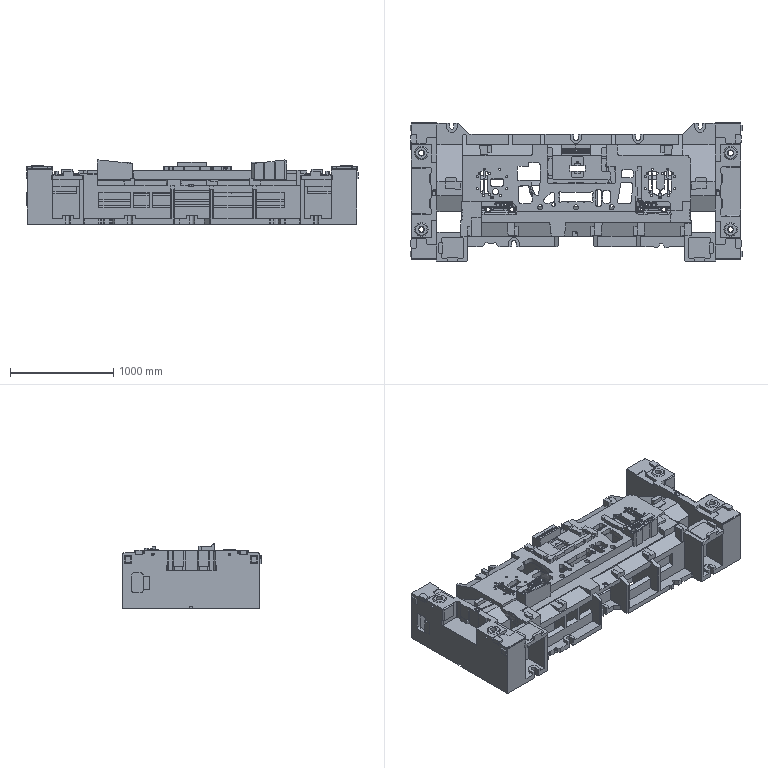Part | NX | features solid 2 | 1 solid | 1591 faces | box 3210 x 1335 x 620.436 mm | volume 634176186 mm3 | plane 1078 | spline 383 | cylinder 123 | cone 7 | commonest cylinder face diameters 20 x22 40 x16 18 x14 50 x12 30 x11 100 x8